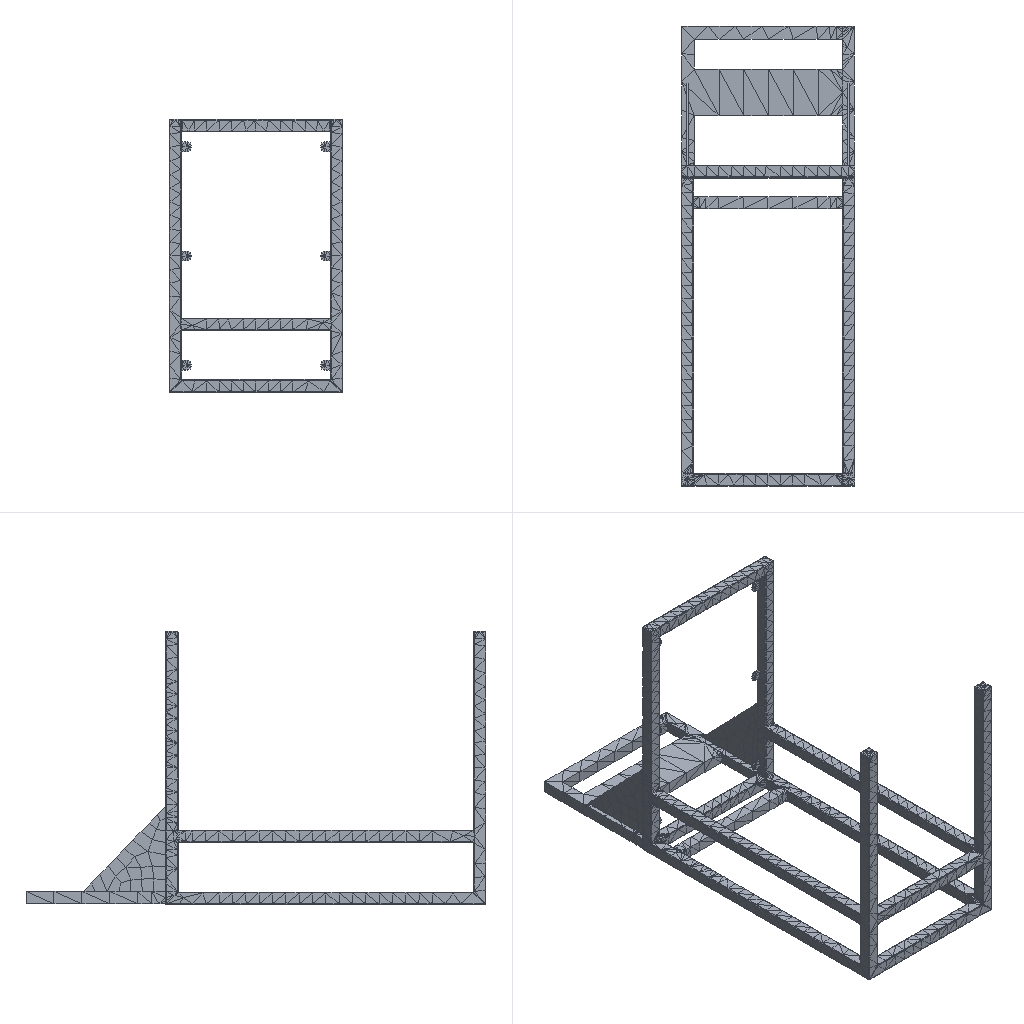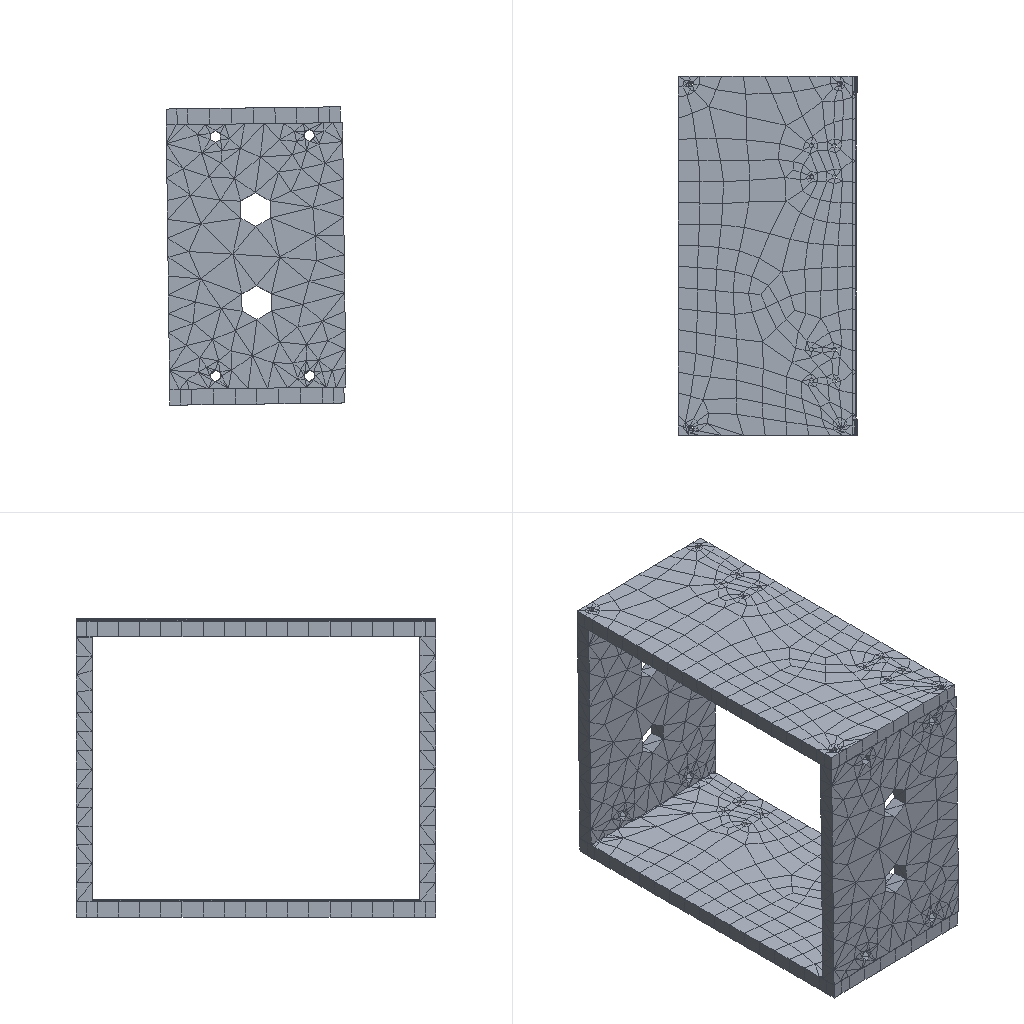Simulation study | ansys workbench
Set-up summary:
category,name,step,type,value,unit,region
solver,ansys_mapdl
solver,version,,,22.1
solver,version,,,22.1
units,MPA,,stated
analysis,deck1,,static,static
load_step,requested,,,1
analysis,nlgeom,,,False
mesh,nodes,,,10998
mesh,elements,,,4846
element_type,ANSYS 186 (type 1),,solid,298
element_type,ANSYS 187 (type 2),,solid,1567
element_type,ANSYS 187 (type 3),,solid,1567
element_type,ANSYS 186 (type 4),,solid,298
element_type,ANSYS 174 (type 5),,contact,96
element_type,ANSYS 170 (type 6),,target,96
element_type,ANSYS 174 (type 7),,contact,80
element_type,ANSYS 170 (type 8),,target,80
element_type,ANSYS 174 (type 9),,contact,100
element_type,ANSYS 170 (type 10),,target,100
element_type,ANSYS 174 (type 11),,contact,84
element_type,ANSYS 170 (type 12),,target,84
element_type,ANSYS 154 (type 13),,surface,396
load,load commands in deck,,count,3
bc,support commands in deck,,count,1
named_set,_FIXEDSU,,component
analysis,deck2,,static,static
load_step,requested,,,1
analysis,nlgeom,,,False
mesh,nodes,,,26590
mesh,elements,,,14360
element_type,ANSYS 186 (type 1),,solid,31
element_type,ANSYS 186 (type 2),,solid,25
element_type,ANSYS 187 (type 3),,solid,13867
element_type,ANSYS 174 (type 4),,contact,57
element_type,ANSYS 170 (type 5),,target,57
element_type,ANSYS 174 (type 6),,contact,50
element_type,ANSYS 170 (type 7),,target,50
element_type,ANSYS 154 (type 8),,surface,223
load,load commands in deck,,count,3
bc,support commands in deck,,count,1
named_set,_FIXEDSU,,component
material,1,,in results
material,2,,in results
material,3,,in results
material,4,,in results
material,1,,in results
material,2,,in results
material,3,,in results
check,setup vs results,,match,396 surface effect element(s) are not in the reader's mesh and were not compared
check,setup vs results,,match,223 surface effect element(s) are not in the reader's mesh and were not compared
Results summary:
result,analysis,,,static
result,last_loadstep,,,1
result,primary field,,,displacement
result,reaction total,1,FX,-0.0,N
result,reaction total,1,FY,50000.0,N
result,reaction total,1,FZ,2e-06,N
result,mass,,,0.1299,"NMM: mm, ton, N, s, mV, mA, degC"
result,analysis,,,static
result,last_loadstep,,,1
result,primary field,,,displacement
result,reaction total,1,FX,-0.0,N
result,reaction total,1,FY,-6e-06,N
result,reaction total,1,FZ,-50000,N
result,mass,,,0.1635,"NMM: mm, ton, N, s, mV, mA, degC"